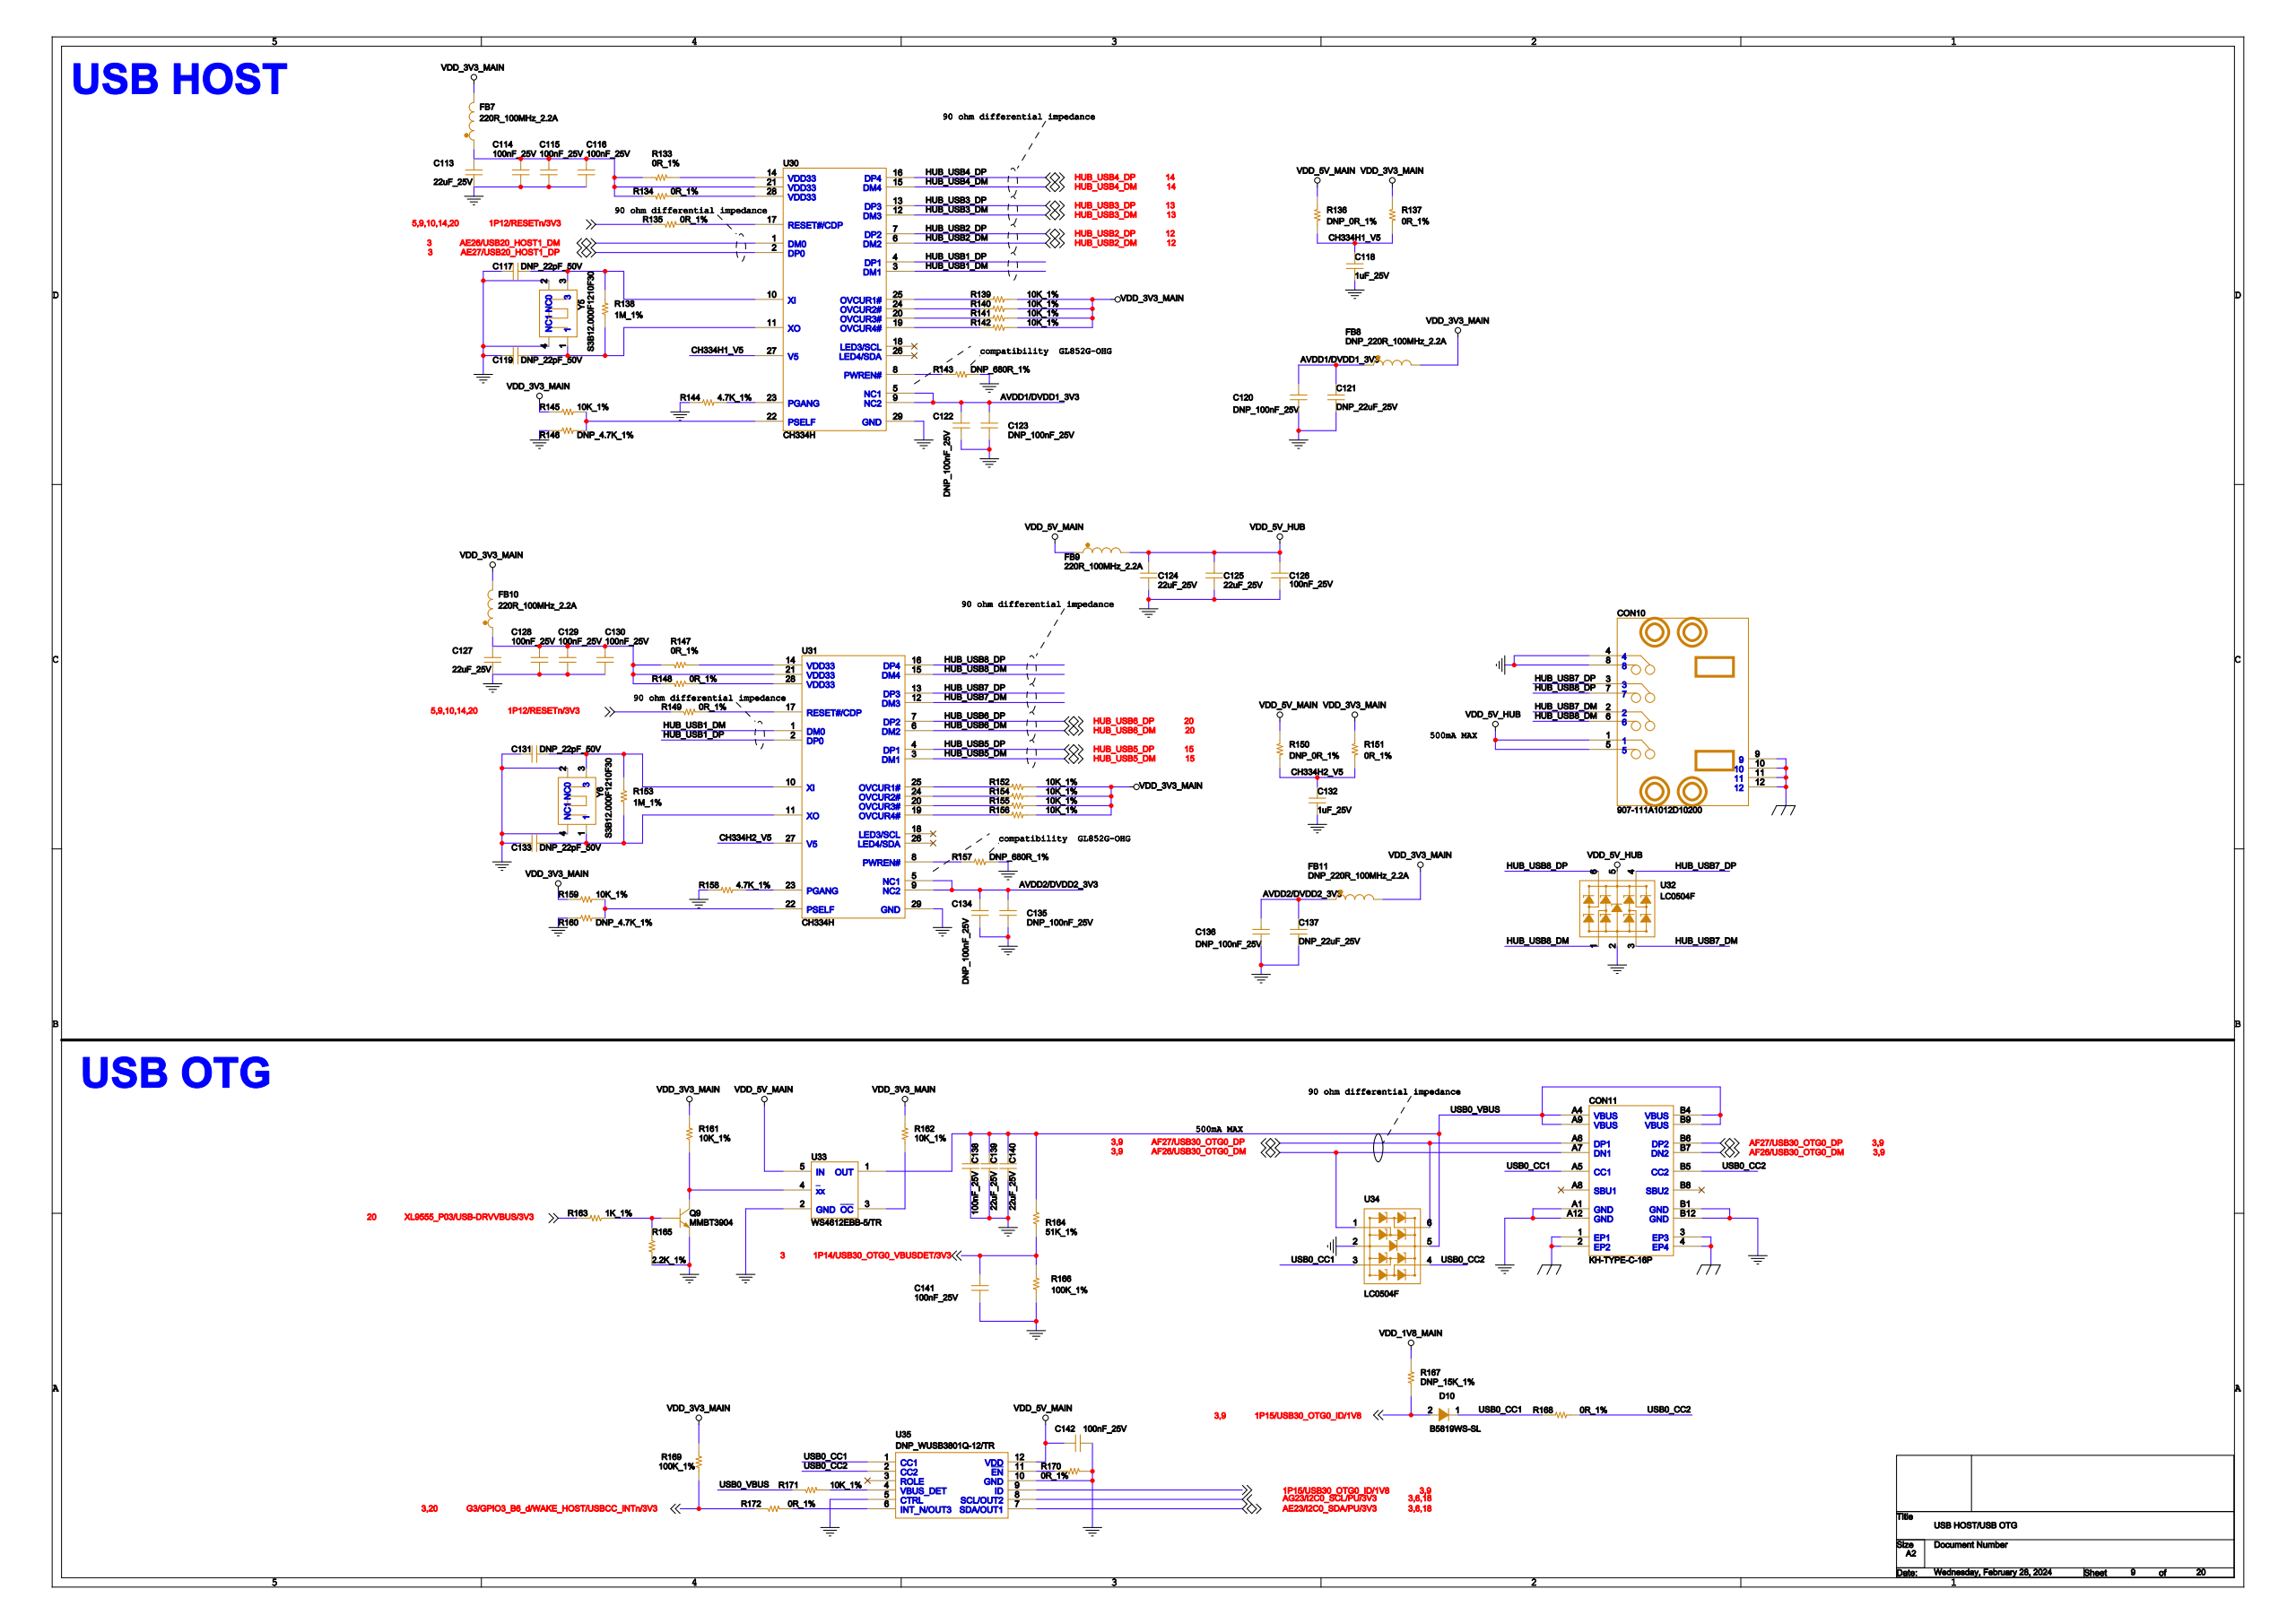Circuit board | Cadence Allegro | 1024 parts | 682 nets | one sheet of the schematic
Parts on this sheet (reference | value | footprint):
C113 | 22uF_25V | C0805
C114 | 100nF_25V | C0402
C115 | 100nF_25V | C0402
C116 | 100nF_25V | C0402
C117 | DNP_22pF_50V | C0603
C118 | 1uF_25V | C0603
C119 | DNP_22pF_50V | C0603
C120 | DNP_100nF_25V | C0402
C121 | DNP_22uF_25V | C0805
C123 | DNP_100nF_25V | C0402
C124 | 22uF_25V | C0805
C125 | 22uF_25V | C0805
C126 | 100nF_25V | C0402
C127 | 22uF_25V | C0805
C128 | 100nF_25V | C0402
C129 | 100nF_25V | C0402
C130 | 100nF_25V | C0402
C131 | DNP_22pF_50V | C0603
C132 | 1uF_25V | C0603
C133 | DNP_22pF_50V | C0603
C135 | DNP_100nF_25V | C0402
C136 | DNP_100nF_25V | C0402
C137 | DNP_22uF_25V | C0805
C138 | 100nF_25V | C0402
C139 | 22uF_25V | C0805
C140 | 22uF_25V | C0805
C141 | 100nF_25V | C0402
C142 | 100nF_25V | C0402
CON10 | FUS208-FDBW3K | CON_USBA_DUAL
CON11 | KH-TYPE-C-16P | TYPE-C_16P_90_SMD
D10 | B5819WS-SL | SOD-323
FB7 | 220R_100MHz_2A | L0603
FB8 | DNP_220R_100MHz_2A | L0603
FB9 | 220R_100MHz_2A | L0603
FB10 | 220R_100MHz_2A | L0603
FB11 | DNP_220R_100MHz_2A | L0603
Q9 | MMBT3904 | SOT23-3_DBZ3
R133 | 0R_1% | R0402
R134 | 0R_1% | R0402
R135 | 0R_1% | R0402
R136 | DNP_0R_1% | R0603
R137 | 0R_1% | R0603
R138 | 1M_1% | R0603
R139 | 10K_1% | R0402
R140 | 10K_1% | R0402
R141 | 10K_1% | R0402
R142 | 10K_1% | R0402
R143 | DNP_680R_1% | R0603
R144 | 4.7K_1% | R0402
R145 | 10K_1% | R0402
R146 | DNP_4.7K_1% | R0402
R147 | 0R_1% | R0402
R148 | 0R_1% | R0402
R149 | 0R_1% | R0402
R150 | DNP_0R_1% | R0603
R151 | 0R_1% | R0603
R152 | 10K_1% | R0402
R153 | 1M_1% | R0603
R154 | 10K_1% | R0402
R155 | 10K_1% | R0402
R156 | 10K_1% | R0402
R157 | DNP_680R_1% | R0603
R158 | 4.7K_1% | R0402
R159 | 10K_1% | R0402
R160 | DNP_4.7K_1% | R0402
R161 | 10K_1% | R0402
R162 | 10K_1% | R0402
R163 | 1K_1% | R0402
R164 | 51K_1% | R0402
R165 | 2.2K_1% | R0603
R166 | 100K_1% | R0402
R167 | DNP_15K_1% | R0402
R168 | 0R_1% | R0402
R169 | 100K_1% | R0402
R170 | 0R_1% | R0402
R171 | 10K_1% | R0402
R172 | 0R_1% | R0402
U30 | CH334H | QFN28_5X5
U31 | CH334H | QFN28_5X5
U32 | LC0504F | SOT363
U33 | WS4612EBB-5/TR | SOT23-5
U34 | LC0504F | SOT363
U35 | DNP_WUSB3801Q-12/TR | QFN1616-12L
Y5 | S3B12.000F1210F30 | SMD_3225
Y6 | S3B12.000F1210F30 | SMD_3225
Nets of these parts (net: part-pin ...):
HUB_USB5_DP: U31-4
HUB_USB5_DM: U31-3
GND: C113-2 C114-2 C115-2 C116-2 C117-1 C118-2 C119-1 C120-2 C121-2 C123-2 C124-2 C125-2 C126-2 C127-2 C128-2 C129-2 C130-2 C131-1 C132-2 C133-1 C135-2 C136-2 C137-2 C138-2 C139-2 C140-2 C141-2 C142-2 CON10-4 CON10-8 CON11-A1 CON11-A12 CON11-B1 CON11-B12 Q9-2 R143-2 R144-2 R146-2 R157-2 R158-2 R160-2 R165-1 R166-1 R170-1 U32-2 U33-2 U34-2 U35-5 U35-10 Y5-2 Y5-4 Y6-2 Y6-4 U30-29 U31-29
VDD_5V_MAIN: C142-1 FB9-1 R136-2 R150-2 U33-5 U35-12
VDD_1V8_MAIN: R167-1
EGND: CON10-9 CON10-10 CON10-11 CON10-12 CON11-1 CON11-2 CON11-3 CON11-4
VDD_3V3_MAIN: FB7-2 FB8-2 FB10-2 FB11-2 R137-2 R139-2 R140-2 R141-2 R142-2 R145-1 R151-2 R152-2 R154-2 R155-2 R156-2 R159-1 R161-1 R162-2 R169-1
1P12/RESETN/3V3: R135-2 R149-2
1P15/USB30_OTG0_ID/1V8: D10-2 R167-2 U35-9
AE27/USB20_HOST1_DP: U30-2
AE26/USB20_HOST1_DM: U30-1
AF27/USB30_OTG0_DP: CON11-A6 CON11-B6 U34-6
AF26/USB30_OTG0_DM: CON11-A7 CON11-B7 U34-1
1P14/USB30_OTG0_VBUSDET/3V3: C141-1 R164-1 R166-2
AE23/I2C0_SDA/PU/3V3: U35-7
AG23/I2C0_SCL/PU/3V3: U35-8
G3/GPIO3_B6_D/WAKE_HOST/USBCC_I: R169-2 R172-2
VDD_5V_HUB: C124-1 C125-1 C126-1 CON10-1 CON10-5 FB9-2 U32-5
HUB_USB7_DM: CON10-2 U32-3 U31-12
HUB_USB7_DP: CON10-3 U32-4 U31-13
HUB_USB8_DM: CON10-6 U32-1 U31-15
HUB_USB8_DP: CON10-7 U32-6 U31-16
USB0_CC1: CON11-A5 D10-1 R168-2 U34-3 U35-1
USB0_CC2: CON11-B5 R168-1 U34-4 U35-2
USB0_VBUS: C138-1 C139-1 C140-1 CON11-A4 CON11-A9 CON11-B4 CON11-B9 R164-2 R171-2 U33-1 U34-5
N21626444: Q9-1 R163-1 R165-2
XL9555_P03/USB-DRVVBUS/3V3: R163-2
N21625946: Q9-3 R161-2 U33-4
N21625934: R162-1 U33-3
N21626246: R171-1 U35-4
CH334H1_V5: C118-1 R136-1 R137-1 U30-27
CH334H2_V5: C132-1 R150-1 R151-1 U31-27
N21681597: R144-1 U30-23
N21624822: R158-1 U31-23
N21681617: R145-2 R146-1 U30-22
N21624834: R159-2 R160-1 U31-22
N21626181: R170-2 U35-11
N21625887: R172-1 U35-6
HUB_USB2_DM: U30-6
HUB_USB2_DP: U30-7
HUB_USB3_DM: U30-12
HUB_USB3_DP: U30-13
N21681223: C113-1 C114-1 C115-1 C116-1 FB7-1 R133-1 R134-1 U30-21
N21681243: R133-2 U30-14
N21681482: R134-2 U30-28
N21681326: R135-1 U30-17
N21624416: C127-1 C128-1 C129-1 C130-1 FB10-1 R147-1 R148-1 U31-21
N21624444: R147-2 U31-14
N21624519: R149-1 U31-17
N21624705: R148-2 U31-28
AVDD1/DVDD1_3V3: C120-1 C121-1 C123-1 FB8-1 U30-5 U30-9
AVDD2/DVDD2_3V3: C135-1 C136-1 C137-1 FB11-1 U31-5 U31-9
N21681201: R143-1 U30-8
N21624394: R157-1 U31-8
HUB_USB4_DP: U30-16
HUB_USB4_DM: U30-15
N21624716: C131-2 R153-1 Y6-3 U31-10
N21624710: C133-2 R153-2 Y6-1 U31-11
N21681488: C117-2 R138-1 Y5-3 U30-10
N21681484: C119-2 R138-2 Y5-1 U30-11
HUB_USB6_DM: U31-6
HUB_USB6_DP: U31-7
N21681429: R139-1 U30-25
N21681431: R140-1 U30-24
N21681413: R141-1 U30-20
N21681415: R142-1 U30-19
N21624648: R152-1 U31-25
N21624650: R154-1 U31-24
N21624630: R155-1 U31-20
N21624632: R156-1 U31-19
HUB_USB1_DM: U30-3 U31-1
HUB_USB1_DP: U30-4 U31-2